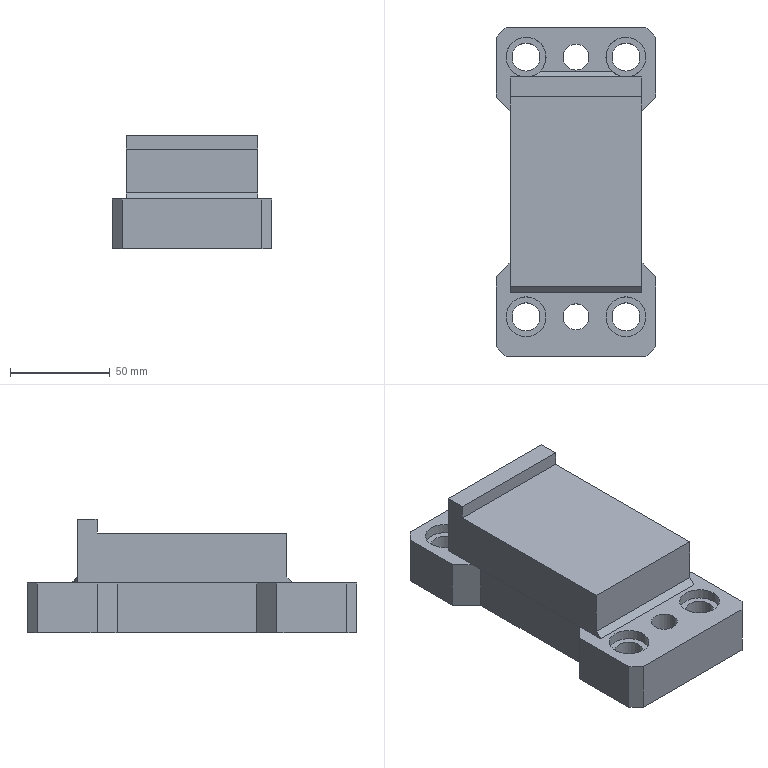Part | NX | features solid 2 | 1 solid | 44 faces | box 80 x 165 x 57 mm | volume 441871 mm3 | plane 34 | cylinder 10 | commonest cylinder face diameters 14 x4 20 x4 13 x2
STEP:
#1=CARTESIAN_POINT('',(-250.,-747.,-70.));
#2=VERTEX_POINT('',#1);
#3=CARTESIAN_POINT('',(-180.,-747.,-70.));
#4=VERTEX_POINT('',#3);
#5=CARTESIAN_POINT('',(-215.,-747.,-70.));
#6=DIRECTION('',(1.,0.,0.));
#7=VECTOR('',#6,1000.);
#8=LINE('',#5,#7);
#9=EDGE_CURVE('',#2,#4,#8,.T.);
#10=ORIENTED_EDGE('',*,*,#9,.T.);
#11=CARTESIAN_POINT('',(-175.,-742.,-70.));
#12=VERTEX_POINT('',#11);
#13=CARTESIAN_POINT('',(-156.25,-723.25,-70.));
#14=DIRECTION('',(0.7071,0.7071,0.));
#15=VECTOR('',#14,1000.);
#16=LINE('',#13,#15);
#17=EDGE_CURVE('',#12,#4,#16,.F.);
#18=ORIENTED_EDGE('',*,*,#17,.F.);
#19=CARTESIAN_POINT('',(-175.,-707.,-70.));
#20=VERTEX_POINT('',#19);
#21=CARTESIAN_POINT('',(-175.,-664.5,-70.));
#22=DIRECTION('',(0.,1.,0.));
#23=VECTOR('',#22,1000.);
#24=LINE('',#21,#23);
#25=EDGE_CURVE('',#12,#20,#24,.T.);
#26=ORIENTED_EDGE('',*,*,#25,.T.);
#27=CARTESIAN_POINT('',(-182.,-700.,-70.));
#28=VERTEX_POINT('',#27);
#29=CARTESIAN_POINT('',(-175.,-707.,-70.));
#30=DIRECTION('',(-0.7071,0.7071,0.));
#31=VECTOR('',#30,1000.);
#32=LINE('',#29,#31);
#33=EDGE_CURVE('',#20,#28,#32,.T.);
#34=ORIENTED_EDGE('',*,*,#33,.T.);
#35=CARTESIAN_POINT('',(-182.,-715.,-70.));
#36=VERTEX_POINT('',#35);
#37=CARTESIAN_POINT('',(-182.,-712.,-70.));
#38=DIRECTION('',(0.,1.,0.));
#39=VECTOR('',#38,1000.);
#40=LINE('',#37,#39);
#41=EDGE_CURVE('',#36,#28,#40,.T.);
#42=ORIENTED_EDGE('',*,*,#41,.F.);
#43=CARTESIAN_POINT('',(-248.,-715.,-70.));
#44=VERTEX_POINT('',#43);
#45=CARTESIAN_POINT('',(-182.,-715.,-70.));
#46=DIRECTION('',(1.,0.,0.));
#47=VECTOR('',#46,1000.);
#48=LINE('',#45,#47);
#49=EDGE_CURVE('',#44,#36,#48,.T.);
#50=ORIENTED_EDGE('',*,*,#49,.F.);
#51=CARTESIAN_POINT('',(-248.,-700.,-70.));
#52=VERTEX_POINT('',#51);
#53=CARTESIAN_POINT('',(-248.,-712.,-70.));
#54=DIRECTION('',(0.,1.,0.));
#55=VECTOR('',#54,1000.);
#56=LINE('',#53,#55);
#57=EDGE_CURVE('',#44,#52,#56,.T.);
#58=ORIENTED_EDGE('',*,*,#57,.T.);
#59=CARTESIAN_POINT('',(-255.,-707.,-70.));
#60=VERTEX_POINT('',#59);
#61=CARTESIAN_POINT('',(-245.,-697.,-70.));
#62=DIRECTION('',(-0.7071,-0.7071,0.));
#63=VECTOR('',#62,1000.);
#64=LINE('',#61,#63);
#65=EDGE_CURVE('',#52,#60,#64,.T.);
#66=ORIENTED_EDGE('',*,*,#65,.T.);
#67=CARTESIAN_POINT('',(-255.,-742.,-70.));
#68=VERTEX_POINT('',#67);
#69=CARTESIAN_POINT('',(-255.,-664.5,-70.));
#70=DIRECTION('',(0.,-1.,0.));
#71=VECTOR('',#70,1000.);
#72=LINE('',#69,#71);
#73=EDGE_CURVE('',#60,#68,#72,.T.);
#74=ORIENTED_EDGE('',*,*,#73,.T.);
#75=CARTESIAN_POINT('',(-273.75,-723.25,-70.));
#76=DIRECTION('',(0.7071,-0.7071,0.));
#77=VECTOR('',#76,1000.);
#78=LINE('',#75,#77);
#79=EDGE_CURVE('',#2,#68,#78,.F.);
#80=ORIENTED_EDGE('',*,*,#79,.F.);
#81=EDGE_LOOP('',(#10,#18,#26,#34,#42,#50,#58,#66,#74,#80));
#82=FACE_BOUND('',#81,.T.);
#83=CARTESIAN_POINT('',(-190.,-717.,-70.));
#84=VERTEX_POINT('',#83);
#85=CARTESIAN_POINT('',(-190.,-727.,-70.));
#86=DIRECTION('',(0.,0.,-1.));
#87=DIRECTION('',(0.,1.,0.));
#88=AXIS2_PLACEMENT_3D('',#85,#86,#87);
#89=CIRCLE('',#88,10.);
#90=EDGE_CURVE('',#84,#84,#89,.T.);
#91=ORIENTED_EDGE('',*,*,#90,.T.);
#92=EDGE_LOOP('',(#91));
#93=FACE_BOUND('',#92,.T.);
#94=CARTESIAN_POINT('',(-215.,-720.5,-70.));
#95=VERTEX_POINT('',#94);
#96=CARTESIAN_POINT('',(-215.,-727.,-70.));
#97=DIRECTION('',(0.,0.,-1.));
#98=DIRECTION('',(0.,1.,0.));
#99=AXIS2_PLACEMENT_3D('',#96,#97,#98);
#100=CIRCLE('',#99,6.5);
#101=EDGE_CURVE('',#95,#95,#100,.T.);
#102=ORIENTED_EDGE('',*,*,#101,.T.);
#103=EDGE_LOOP('',(#102));
#104=FACE_BOUND('',#103,.T.);
#105=CARTESIAN_POINT('',(-240.,-717.,-70.));
#106=VERTEX_POINT('',#105);
#107=CARTESIAN_POINT('',(-240.,-727.,-70.));
#108=DIRECTION('',(0.,0.,-1.));
#109=DIRECTION('',(0.,1.,0.));
#110=AXIS2_PLACEMENT_3D('',#107,#108,#109);
#111=CIRCLE('',#110,10.);
#112=EDGE_CURVE('',#106,#106,#111,.T.);
#113=ORIENTED_EDGE('',*,*,#112,.T.);
#114=EDGE_LOOP('',(#113));
#115=FACE_BOUND('',#114,.T.);
#116=CARTESIAN_POINT('',(-215.,-664.5,-70.));
#117=DIRECTION('',(0.,0.,1.));
#118=DIRECTION('',(0.,1.,0.));
#119=AXIS2_PLACEMENT_3D('',#116,#117,#118);
#120=PLANE('',#119);
#121=ADVANCED_FACE('',(#82,#93,#104,#115),#120,.T.);
#122=CARTESIAN_POINT('',(-180.,-582.,-70.));
#123=VERTEX_POINT('',#122);
#124=CARTESIAN_POINT('',(-250.,-582.,-70.));
#125=VERTEX_POINT('',#124);
#126=CARTESIAN_POINT('',(-215.,-582.,-70.));
#127=DIRECTION('',(-1.,0.,0.));
#128=VECTOR('',#127,1000.);
#129=LINE('',#126,#128);
#130=EDGE_CURVE('',#123,#125,#129,.T.);
#131=ORIENTED_EDGE('',*,*,#130,.T.);
#132=CARTESIAN_POINT('',(-255.,-587.,-70.));
#133=VERTEX_POINT('',#132);
#134=CARTESIAN_POINT('',(-273.75,-605.75,-70.));
#135=DIRECTION('',(-0.7071,-0.7071,0.));
#136=VECTOR('',#135,1000.);
#137=LINE('',#134,#136);
#138=EDGE_CURVE('',#133,#125,#137,.F.);
#139=ORIENTED_EDGE('',*,*,#138,.F.);
#140=CARTESIAN_POINT('',(-255.,-617.,-70.));
#141=VERTEX_POINT('',#140);
#142=CARTESIAN_POINT('',(-255.,-664.5,-70.));
#143=DIRECTION('',(0.,-1.,0.));
#144=VECTOR('',#143,1000.);
#145=LINE('',#142,#144);
#146=EDGE_CURVE('',#133,#141,#145,.T.);
#147=ORIENTED_EDGE('',*,*,#146,.T.);
#148=CARTESIAN_POINT('',(-248.,-624.,-70.));
#149=VERTEX_POINT('',#148);
#150=CARTESIAN_POINT('',(-245.,-627.,-70.));
#151=DIRECTION('',(-0.7071,0.7071,0.));
#152=VECTOR('',#151,1000.);
#153=LINE('',#150,#152);
#154=EDGE_CURVE('',#149,#141,#153,.T.);
#155=ORIENTED_EDGE('',*,*,#154,.F.);
#156=CARTESIAN_POINT('',(-248.,-607.,-70.));
#157=VERTEX_POINT('',#156);
#158=CARTESIAN_POINT('',(-248.,-712.,-70.));
#159=DIRECTION('',(0.,1.,0.));
#160=VECTOR('',#159,1000.);
#161=LINE('',#158,#160);
#162=EDGE_CURVE('',#149,#157,#161,.T.);
#163=ORIENTED_EDGE('',*,*,#162,.T.);
#164=CARTESIAN_POINT('',(-240.,-607.,-70.));
#165=VERTEX_POINT('',#164);
#166=CARTESIAN_POINT('',(-182.,-607.,-70.));
#167=DIRECTION('',(-1.,0.,0.));
#168=VECTOR('',#167,1000.);
#169=LINE('',#166,#168);
#170=EDGE_CURVE('',#165,#157,#169,.T.);
#171=ORIENTED_EDGE('',*,*,#170,.F.);
#172=CARTESIAN_POINT('',(-232.859,-604.,-70.));
#173=VERTEX_POINT('',#172);
#174=CARTESIAN_POINT('',(-240.,-597.,-70.));
#175=DIRECTION('',(0.,0.,-1.));
#176=DIRECTION('',(0.,1.,0.));
#177=AXIS2_PLACEMENT_3D('',#174,#175,#176);
#178=CIRCLE('',#177,10.);
#179=EDGE_CURVE('',#165,#173,#178,.T.);
#180=ORIENTED_EDGE('',*,*,#179,.T.);
#181=CARTESIAN_POINT('',(-197.141,-604.,-70.));
#182=VERTEX_POINT('',#181);
#183=CARTESIAN_POINT('',(-240.,-604.,-70.));
#184=DIRECTION('',(-1.,0.,0.));
#185=VECTOR('',#184,1000.);
#186=LINE('',#183,#185);
#187=EDGE_CURVE('',#182,#173,#186,.T.);
#188=ORIENTED_EDGE('',*,*,#187,.F.);
#189=CARTESIAN_POINT('',(-190.,-607.,-70.));
#190=VERTEX_POINT('',#189);
#191=CARTESIAN_POINT('',(-190.,-597.,-70.));
#192=DIRECTION('',(0.,0.,-1.));
#193=DIRECTION('',(0.,1.,0.));
#194=AXIS2_PLACEMENT_3D('',#191,#192,#193);
#195=CIRCLE('',#194,10.);
#196=EDGE_CURVE('',#182,#190,#195,.T.);
#197=ORIENTED_EDGE('',*,*,#196,.T.);
#198=CARTESIAN_POINT('',(-182.,-607.,-70.));
#199=VERTEX_POINT('',#198);
#200=CARTESIAN_POINT('',(-182.,-607.,-70.));
#201=DIRECTION('',(-1.,0.,0.));
#202=VECTOR('',#201,1000.);
#203=LINE('',#200,#202);
#204=EDGE_CURVE('',#199,#190,#203,.T.);
#205=ORIENTED_EDGE('',*,*,#204,.F.);
#206=CARTESIAN_POINT('',(-182.,-624.,-70.));
#207=VERTEX_POINT('',#206);
#208=CARTESIAN_POINT('',(-182.,-712.,-70.));
#209=DIRECTION('',(0.,1.,0.));
#210=VECTOR('',#209,1000.);
#211=LINE('',#208,#210);
#212=EDGE_CURVE('',#207,#199,#211,.T.);
#213=ORIENTED_EDGE('',*,*,#212,.F.);
#214=CARTESIAN_POINT('',(-175.,-617.,-70.));
#215=VERTEX_POINT('',#214);
#216=CARTESIAN_POINT('',(-175.,-617.,-70.));
#217=DIRECTION('',(-0.7071,-0.7071,0.));
#218=VECTOR('',#217,1000.);
#219=LINE('',#216,#218);
#220=EDGE_CURVE('',#215,#207,#219,.T.);
#221=ORIENTED_EDGE('',*,*,#220,.F.);
#222=CARTESIAN_POINT('',(-175.,-587.,-70.));
#223=VERTEX_POINT('',#222);
#224=CARTESIAN_POINT('',(-175.,-664.5,-70.));
#225=DIRECTION('',(0.,1.,0.));
#226=VECTOR('',#225,1000.);
#227=LINE('',#224,#226);
#228=EDGE_CURVE('',#215,#223,#227,.T.);
#229=ORIENTED_EDGE('',*,*,#228,.T.);
#230=CARTESIAN_POINT('',(-156.25,-605.75,-70.));
#231=DIRECTION('',(-0.7071,0.7071,0.));
#232=VECTOR('',#231,1000.);
#233=LINE('',#230,#232);
#234=EDGE_CURVE('',#123,#223,#233,.F.);
#235=ORIENTED_EDGE('',*,*,#234,.F.);
#236=EDGE_LOOP('',(#131,#139,#147,#155,#163,#171,#180,#188,#197,#205,#213,#221,#229,#235));
#237=FACE_BOUND('',#236,.T.);
#238=CARTESIAN_POINT('',(-215.,-590.5,-70.));
#239=VERTEX_POINT('',#238);
#240=CARTESIAN_POINT('',(-215.,-597.,-70.));
#241=DIRECTION('',(0.,0.,-1.));
#242=DIRECTION('',(0.,1.,0.));
#243=AXIS2_PLACEMENT_3D('',#240,#241,#242);
#244=CIRCLE('',#243,6.5);
#245=EDGE_CURVE('',#239,#239,#244,.T.);
#246=ORIENTED_EDGE('',*,*,#245,.T.);
#247=EDGE_LOOP('',(#246));
#248=FACE_BOUND('',#247,.T.);
#249=CARTESIAN_POINT('',(-215.,-664.5,-70.));
#250=DIRECTION('',(0.,0.,1.));
#251=DIRECTION('',(0.,1.,0.));
#252=AXIS2_PLACEMENT_3D('',#249,#250,#251);
#253=PLANE('',#252);
#254=ADVANCED_FACE('',(#237,#248),#253,.T.);
#255=CARTESIAN_POINT('',(-190.,-720.,-95.));
#256=VERTEX_POINT('',#255);
#257=CARTESIAN_POINT('',(-190.,-727.,-95.));
#258=DIRECTION('',(0.,0.,-1.));
#259=DIRECTION('',(0.,1.,0.));
#260=AXIS2_PLACEMENT_3D('',#257,#258,#259);
#261=CIRCLE('',#260,7.);
#262=EDGE_CURVE('',#256,#256,#261,.T.);
#263=ORIENTED_EDGE('',*,*,#262,.T.);
#264=EDGE_LOOP('',(#263));
#265=FACE_BOUND('',#264,.T.);
#266=CARTESIAN_POINT('',(-190.,-734.,-75.));
#267=VERTEX_POINT('',#266);
#268=CARTESIAN_POINT('',(-190.,-727.,-75.));
#269=DIRECTION('',(0.,0.,-1.));
#270=DIRECTION('',(0.,-1.,0.));
#271=AXIS2_PLACEMENT_3D('',#268,#269,#270);
#272=CIRCLE('',#271,7.);
#273=EDGE_CURVE('',#267,#267,#272,.T.);
#274=ORIENTED_EDGE('',*,*,#273,.F.);
#275=EDGE_LOOP('',(#274));
#276=FACE_BOUND('',#275,.T.);
#277=CARTESIAN_POINT('',(-190.,-727.,-70.));
#278=DIRECTION('',(0.,0.,-1.));
#279=DIRECTION('',(1.,0.,0.));
#280=AXIS2_PLACEMENT_3D('',#277,#278,#279);
#281=CYLINDRICAL_SURFACE('',#280,7.);
#282=ADVANCED_FACE('',(#265,#276),#281,.F.);
#283=CARTESIAN_POINT('',(-240.,-720.,-95.));
#284=VERTEX_POINT('',#283);
#285=CARTESIAN_POINT('',(-240.,-727.,-95.));
#286=DIRECTION('',(0.,0.,-1.));
#287=DIRECTION('',(0.,1.,0.));
#288=AXIS2_PLACEMENT_3D('',#285,#286,#287);
#289=CIRCLE('',#288,7.);
#290=EDGE_CURVE('',#284,#284,#289,.T.);
#291=ORIENTED_EDGE('',*,*,#290,.T.);
#292=EDGE_LOOP('',(#291));
#293=FACE_BOUND('',#292,.T.);
#294=CARTESIAN_POINT('',(-240.,-734.,-75.));
#295=VERTEX_POINT('',#294);
#296=CARTESIAN_POINT('',(-240.,-727.,-75.));
#297=DIRECTION('',(0.,0.,-1.));
#298=DIRECTION('',(0.,-1.,0.));
#299=AXIS2_PLACEMENT_3D('',#296,#297,#298);
#300=CIRCLE('',#299,7.);
#301=EDGE_CURVE('',#295,#295,#300,.T.);
#302=ORIENTED_EDGE('',*,*,#301,.F.);
#303=EDGE_LOOP('',(#302));
#304=FACE_BOUND('',#303,.T.);
#305=CARTESIAN_POINT('',(-240.,-727.,-70.));
#306=DIRECTION('',(0.,0.,-1.));
#307=DIRECTION('',(1.,0.,0.));
#308=AXIS2_PLACEMENT_3D('',#305,#306,#307);
#309=CYLINDRICAL_SURFACE('',#308,7.);
#310=ADVANCED_FACE('',(#293,#304),#309,.F.);
#311=CARTESIAN_POINT('',(-240.,-590.,-95.));
#312=VERTEX_POINT('',#311);
#313=CARTESIAN_POINT('',(-240.,-597.,-95.));
#314=DIRECTION('',(0.,0.,-1.));
#315=DIRECTION('',(0.,1.,0.));
#316=AXIS2_PLACEMENT_3D('',#313,#314,#315);
#317=CIRCLE('',#316,7.);
#318=EDGE_CURVE('',#312,#312,#317,.T.);
#319=ORIENTED_EDGE('',*,*,#318,.T.);
#320=EDGE_LOOP('',(#319));
#321=FACE_BOUND('',#320,.T.);
#322=CARTESIAN_POINT('',(-240.,-604.,-75.));
#323=VERTEX_POINT('',#322);
#324=CARTESIAN_POINT('',(-240.,-597.,-75.));
#325=DIRECTION('',(0.,0.,-1.));
#326=DIRECTION('',(0.,-1.,0.));
#327=AXIS2_PLACEMENT_3D('',#324,#325,#326);
#328=CIRCLE('',#327,7.);
#329=EDGE_CURVE('',#323,#323,#328,.T.);
#330=ORIENTED_EDGE('',*,*,#329,.F.);
#331=EDGE_LOOP('',(#330));
#332=FACE_BOUND('',#331,.T.);
#333=CARTESIAN_POINT('',(-240.,-597.,-70.));
#334=DIRECTION('',(0.,0.,-1.));
#335=DIRECTION('',(1.,0.,0.));
#336=AXIS2_PLACEMENT_3D('',#333,#334,#335);
#337=CYLINDRICAL_SURFACE('',#336,7.);
#338=ADVANCED_FACE('',(#321,#332),#337,.F.);
#339=CARTESIAN_POINT('',(-190.,-590.,-95.));
#340=VERTEX_POINT('',#339);
#341=CARTESIAN_POINT('',(-190.,-597.,-95.));
#342=DIRECTION('',(0.,0.,-1.));
#343=DIRECTION('',(0.,1.,0.));
#344=AXIS2_PLACEMENT_3D('',#341,#342,#343);
#345=CIRCLE('',#344,7.);
#346=EDGE_CURVE('',#340,#340,#345,.T.);
#347=ORIENTED_EDGE('',*,*,#346,.T.);
#348=EDGE_LOOP('',(#347));
#349=FACE_BOUND('',#348,.T.);
#350=CARTESIAN_POINT('',(-190.,-604.,-75.));
#351=VERTEX_POINT('',#350);
#352=CARTESIAN_POINT('',(-190.,-597.,-75.));
#353=DIRECTION('',(0.,0.,-1.));
#354=DIRECTION('',(0.,-1.,0.));
#355=AXIS2_PLACEMENT_3D('',#352,#353,#354);
#356=CIRCLE('',#355,7.);
#357=EDGE_CURVE('',#351,#351,#356,.T.);
#358=ORIENTED_EDGE('',*,*,#357,.F.);
#359=EDGE_LOOP('',(#358));
#360=FACE_BOUND('',#359,.T.);
#361=CARTESIAN_POINT('',(-190.,-597.,-70.));
#362=DIRECTION('',(0.,0.,-1.));
#363=DIRECTION('',(1.,0.,0.));
#364=AXIS2_PLACEMENT_3D('',#361,#362,#363);
#365=CYLINDRICAL_SURFACE('',#364,7.);
#366=ADVANCED_FACE('',(#349,#360),#365,.F.);
#367=CARTESIAN_POINT('',(-215.,-720.5,-95.));
#368=VERTEX_POINT('',#367);
#369=CARTESIAN_POINT('',(-215.,-727.,-95.));
#370=DIRECTION('',(0.,0.,-1.));
#371=DIRECTION('',(0.,1.,0.));
#372=AXIS2_PLACEMENT_3D('',#369,#370,#371);
#373=CIRCLE('',#372,6.5);
#374=EDGE_CURVE('',#368,#368,#373,.T.);
#375=ORIENTED_EDGE('',*,*,#374,.F.);
#376=EDGE_LOOP('',(#375));
#377=FACE_BOUND('',#376,.T.);
#378=ORIENTED_EDGE('',*,*,#318,.F.);
#379=EDGE_LOOP('',(#378));
#380=FACE_BOUND('',#379,.T.);
#381=ORIENTED_EDGE('',*,*,#346,.F.);
#382=EDGE_LOOP('',(#381));
#383=FACE_BOUND('',#382,.T.);
#384=CARTESIAN_POINT('',(-175.,-587.,-95.));
#385=VERTEX_POINT('',#384);
#386=CARTESIAN_POINT('',(-175.,-617.,-95.));
#387=VERTEX_POINT('',#386);
#388=CARTESIAN_POINT('',(-175.,-664.5,-95.));
#389=DIRECTION('',(0.,-1.,0.));
#390=VECTOR('',#389,1000.);
#391=LINE('',#388,#390);
#392=EDGE_CURVE('',#385,#387,#391,.T.);
#393=ORIENTED_EDGE('',*,*,#392,.T.);
#394=CARTESIAN_POINT('',(-185.,-627.,-95.));
#395=VERTEX_POINT('',#394);
#396=CARTESIAN_POINT('',(-175.,-617.,-95.));
#397=DIRECTION('',(-0.7071,-0.7071,0.));
#398=VECTOR('',#397,1000.);
#399=LINE('',#396,#398);
#400=EDGE_CURVE('',#387,#395,#399,.T.);
#401=ORIENTED_EDGE('',*,*,#400,.T.);
#402=CARTESIAN_POINT('',(-185.,-697.,-95.));
#403=VERTEX_POINT('',#402);
#404=CARTESIAN_POINT('',(-185.,-697.,-95.));
#405=DIRECTION('',(0.,1.,0.));
#406=VECTOR('',#405,1000.);
#407=LINE('',#404,#406);
#408=EDGE_CURVE('',#403,#395,#407,.T.);
#409=ORIENTED_EDGE('',*,*,#408,.F.);
#410=CARTESIAN_POINT('',(-175.,-707.,-95.));
#411=VERTEX_POINT('',#410);
#412=CARTESIAN_POINT('',(-175.,-707.,-95.));
#413=DIRECTION('',(-0.7071,0.7071,0.));
#414=VECTOR('',#413,1000.);
#415=LINE('',#412,#414);
#416=EDGE_CURVE('',#411,#403,#415,.T.);
#417=ORIENTED_EDGE('',*,*,#416,.F.);
#418=CARTESIAN_POINT('',(-175.,-742.,-95.));
#419=VERTEX_POINT('',#418);
#420=CARTESIAN_POINT('',(-175.,-664.5,-95.));
#421=DIRECTION('',(0.,-1.,0.));
#422=VECTOR('',#421,1000.);
#423=LINE('',#420,#422);
#424=EDGE_CURVE('',#411,#419,#423,.T.);
#425=ORIENTED_EDGE('',*,*,#424,.T.);
#426=CARTESIAN_POINT('',(-180.,-747.,-95.));
#427=VERTEX_POINT('',#426);
#428=CARTESIAN_POINT('',(-156.25,-723.25,-95.));
#429=DIRECTION('',(-0.7071,-0.7071,0.));
#430=VECTOR('',#429,1000.);
#431=LINE('',#428,#430);
#432=EDGE_CURVE('',#427,#419,#431,.F.);
#433=ORIENTED_EDGE('',*,*,#432,.F.);
#434=CARTESIAN_POINT('',(-250.,-747.,-95.));
#435=VERTEX_POINT('',#434);
#436=CARTESIAN_POINT('',(-215.,-747.,-95.));
#437=DIRECTION('',(-1.,0.,0.));
#438=VECTOR('',#437,1000.);
#439=LINE('',#436,#438);
#440=EDGE_CURVE('',#427,#435,#439,.T.);
#441=ORIENTED_EDGE('',*,*,#440,.T.);
#442=CARTESIAN_POINT('',(-255.,-742.,-95.));
#443=VERTEX_POINT('',#442);
#444=CARTESIAN_POINT('',(-273.75,-723.25,-95.));
#445=DIRECTION('',(-0.7071,0.7071,0.));
#446=VECTOR('',#445,1000.);
#447=LINE('',#444,#446);
#448=EDGE_CURVE('',#443,#435,#447,.F.);
#449=ORIENTED_EDGE('',*,*,#448,.F.);
#450=CARTESIAN_POINT('',(-255.,-707.,-95.));
#451=VERTEX_POINT('',#450);
#452=CARTESIAN_POINT('',(-255.,-664.5,-95.));
#453=DIRECTION('',(0.,1.,0.));
#454=VECTOR('',#453,1000.);
#455=LINE('',#452,#454);
#456=EDGE_CURVE('',#443,#451,#455,.T.);
#457=ORIENTED_EDGE('',*,*,#456,.T.);
#458=CARTESIAN_POINT('',(-245.,-697.,-95.));
#459=VERTEX_POINT('',#458);
#460=CARTESIAN_POINT('',(-245.,-697.,-95.));
#461=DIRECTION('',(-0.7071,-0.7071,0.));
#462=VECTOR('',#461,1000.);
#463=LINE('',#460,#462);
#464=EDGE_CURVE('',#459,#451,#463,.T.);
#465=ORIENTED_EDGE('',*,*,#464,.F.);
#466=CARTESIAN_POINT('',(-245.,-627.,-95.));
#467=VERTEX_POINT('',#466);
#468=CARTESIAN_POINT('',(-245.,-697.,-95.));
#469=DIRECTION('',(0.,1.,0.));
#470=VECTOR('',#469,1000.);
#471=LINE('',#468,#470);
#472=EDGE_CURVE('',#459,#467,#471,.T.);
#473=ORIENTED_EDGE('',*,*,#472,.T.);
#474=CARTESIAN_POINT('',(-255.,-617.,-95.));
#475=VERTEX_POINT('',#474);
#476=CARTESIAN_POINT('',(-245.,-627.,-95.));
#477=DIRECTION('',(-0.7071,0.7071,0.));
#478=VECTOR('',#477,1000.);
#479=LINE('',#476,#478);
#480=EDGE_CURVE('',#467,#475,#479,.T.);
#481=ORIENTED_EDGE('',*,*,#480,.T.);
#482=CARTESIAN_POINT('',(-255.,-587.,-95.));
#483=VERTEX_POINT('',#482);
#484=CARTESIAN_POINT('',(-255.,-664.5,-95.));
#485=DIRECTION('',(0.,1.,0.));
#486=VECTOR('',#485,1000.);
#487=LINE('',#484,#486);
#488=EDGE_CURVE('',#475,#483,#487,.T.);
#489=ORIENTED_EDGE('',*,*,#488,.T.);
#490=CARTESIAN_POINT('',(-250.,-582.,-95.));
#491=VERTEX_POINT('',#490);
#492=CARTESIAN_POINT('',(-273.75,-605.75,-95.));
#493=DIRECTION('',(0.7071,0.7071,0.));
#494=VECTOR('',#493,1000.);
#495=LINE('',#492,#494);
#496=EDGE_CURVE('',#491,#483,#495,.F.);
#497=ORIENTED_EDGE('',*,*,#496,.F.);
#498=CARTESIAN_POINT('',(-180.,-582.,-95.));
#499=VERTEX_POINT('',#498);
#500=CARTESIAN_POINT('',(-215.,-582.,-95.));
#501=DIRECTION('',(1.,0.,0.));
#502=VECTOR('',#501,1000.);
#503=LINE('',#500,#502);
#504=EDGE_CURVE('',#491,#499,#503,.T.);
#505=ORIENTED_EDGE('',*,*,#504,.T.);
#506=CARTESIAN_POINT('',(-156.25,-605.75,-95.));
#507=DIRECTION('',(0.7071,-0.7071,0.));
#508=VECTOR('',#507,1000.);
#509=LINE('',#506,#508);
#510=EDGE_CURVE('',#385,#499,#509,.F.);
#511=ORIENTED_EDGE('',*,*,#510,.F.);
#512=EDGE_LOOP('',(#393,#401,#409,#417,#425,#433,#441,#449,#457,#465,#473,#481,#489,#497,#505,#511));
#513=FACE_BOUND('',#512,.T.);
#514=CARTESIAN_POINT('',(-215.,-590.5,-95.));
#515=VERTEX_POINT('',#514);
#516=CARTESIAN_POINT('',(-215.,-597.,-95.));
#517=DIRECTION('',(0.,0.,-1.));
#518=DIRECTION('',(0.,1.,0.));
#519=AXIS2_PLACEMENT_3D('',#516,#517,#518);
#520=CIRCLE('',#519,6.5);
#521=EDGE_CURVE('',#515,#515,#520,.T.);
#522=ORIENTED_EDGE('',*,*,#521,.F.);
#523=EDGE_LOOP('',(#522));
#524=FACE_BOUND('',#523,.T.);
#525=ORIENTED_EDGE('',*,*,#262,.F.);
#526=EDGE_LOOP('',(#525));
#527=FACE_BOUND('',#526,.T.);
#528=ORIENTED_EDGE('',*,*,#290,.F.);
#529=EDGE_LOOP('',(#528));
#530=FACE_BOUND('',#529,.T.);
#531=CARTESIAN_POINT('',(-215.,-664.5,-95.));
#532=DIRECTION('',(0.,0.,-1.));
#533=DIRECTION('',(0.,-1.,0.));
#534=AXIS2_PLACEMENT_3D('',#531,#532,#533);
#535=PLANE('',#534);
#536=ADVANCED_FACE('',(#377,#380,#383,#513,#524,#527,#530),#535,.T.);
#537=ORIENTED_EDGE('',*,*,#73,.F.);
#538=CARTESIAN_POINT('',(-255.,-707.,-70.));
#539=DIRECTION('',(0.,0.,-1.));
#540=VECTOR('',#539,1000.);
#541=LINE('',#538,#540);
#542=EDGE_CURVE('',#60,#451,#541,.T.);
#543=ORIENTED_EDGE('',*,*,#542,.T.);
#544=ORIENTED_EDGE('',*,*,#456,.F.);
#545=CARTESIAN_POINT('',(-255.,-742.,-95.));
#546=DIRECTION('',(0.,0.,-1.));
#547=VECTOR('',#546,1000.);
#548=LINE('',#545,#547);
#549=EDGE_CURVE('',#68,#443,#548,.T.);
#550=ORIENTED_EDGE('',*,*,#549,.F.);
#551=EDGE_LOOP('',(#537,#543,#544,#550));
#552=FACE_BOUND('',#551,.T.);
#553=CARTESIAN_POINT('',(-255.,-664.5,-95.));
#554=DIRECTION('',(-1.,0.,0.));
#555=DIRECTION('',(0.,0.,-1.));
#556=AXIS2_PLACEMENT_3D('',#553,#554,#555);
#557=PLANE('',#556);
#558=ADVANCED_FACE('',(#552),#557,.T.);
#559=ORIENTED_EDGE('',*,*,#424,.F.);
#560=CARTESIAN_POINT('',(-175.,-707.,-70.));
#561=DIRECTION('',(0.,0.,-1.));
#562=VECTOR('',#561,1000.);
#563=LINE('',#560,#562);
#564=EDGE_CURVE('',#20,#411,#563,.T.);
#565=ORIENTED_EDGE('',*,*,#564,.F.);
#566=ORIENTED_EDGE('',*,*,#25,.F.);
#567=CARTESIAN_POINT('',(-175.,-742.,-95.));
#568=DIRECTION('',(0.,0.,1.));
#569=VECTOR('',#568,1000.);
#570=LINE('',#567,#569);
#571=EDGE_CURVE('',#419,#12,#570,.T.);
#572=ORIENTED_EDGE('',*,*,#571,.F.);
#573=EDGE_LOOP('',(#559,#565,#566,#572));
#574=FACE_BOUND('',#573,.T.);
#575=CARTESIAN_POINT('',(-175.,-664.5,-95.));
#576=DIRECTION('',(1.,0.,0.));
#577=DIRECTION('',(0.,0.,1.));
#578=AXIS2_PLACEMENT_3D('',#575,#576,#577);
#579=PLANE('',#578);
#580=ADVANCED_FACE('',(#574),#579,.T.);
#581=ORIENTED_EDGE('',*,*,#488,.F.);
#582=CARTESIAN_POINT('',(-255.,-617.,-70.));
#583=DIRECTION('',(0.,0.,-1.));
#584=VECTOR('',#583,1000.);
#585=LINE('',#582,#584);
#586=EDGE_CURVE('',#141,#475,#585,.T.);
#587=ORIENTED_EDGE('',*,*,#586,.F.);
#588=ORIENTED_EDGE('',*,*,#146,.F.);
#589=CARTESIAN_POINT('',(-255.,-587.,-95.));
#590=DIRECTION('',(0.,0.,1.));
#591=VECTOR('',#590,1000.);
#592=LINE('',#589,#591);
#593=EDGE_CURVE('',#483,#133,#592,.T.);
#594=ORIENTED_EDGE('',*,*,#593,.F.);
#595=EDGE_LOOP('',(#581,#587,#588,#594));
#596=FACE_BOUND('',#595,.T.);
#597=CARTESIAN_POINT('',(-255.,-664.5,-95.));
#598=DIRECTION('',(-1.,0.,0.));
#599=DIRECTION('',(0.,0.,-1.));
#600=AXIS2_PLACEMENT_3D('',#597,#598,#599);
#601=PLANE('',#600);
#602=ADVANCED_FACE('',(#596),#601,.T.);
#603=ORIENTED_EDGE('',*,*,#440,.F.);
#604=CARTESIAN_POINT('',(-180.,-747.,-95.));
#605=DIRECTION('',(0.,0.,-1.));
#606=VECTOR('',#605,1000.);
#607=LINE('',#604,#606);
#608=EDGE_CURVE('',#4,#427,#607,.T.);
#609=ORIENTED_EDGE('',*,*,#608,.F.);
#610=ORIENTED_EDGE('',*,*,#9,.F.);
#611=CARTESIAN_POINT('',(-250.,-747.,-95.));
#612=DIRECTION('',(0.,0.,1.));
#613=VECTOR('',#612,1000.);
#614=LINE('',#611,#613);
#615=EDGE_CURVE('',#435,#2,#614,.T.);
#616=ORIENTED_EDGE('',*,*,#615,.F.);
#617=EDGE_LOOP('',(#603,#609,#610,#616));
#618=FACE_BOUND('',#617,.T.);
#619=CARTESIAN_POINT('',(-215.,-747.,-95.));
#620=DIRECTION('',(0.,-1.,0.));
#621=DIRECTION('',(0.,0.,1.));
#622=AXIS2_PLACEMENT_3D('',#619,#620,#621);
#623=PLANE('',#622);
#624=ADVANCED_FACE('',(#618),#623,.T.);
#625=ORIENTED_EDGE('',*,*,#228,.F.);
#626=CARTESIAN_POINT('',(-175.,-617.,-70.));
#627=DIRECTION('',(0.,0.,-1.));
#628=VECTOR('',#627,1000.);
#629=LINE('',#626,#628);
#630=EDGE_CURVE('',#215,#387,#629,.T.);
#631=ORIENTED_EDGE('',*,*,#630,.T.);
#632=ORIENTED_EDGE('',*,*,#392,.F.);
#633=CARTESIAN_POINT('',(-175.,-587.,-95.));
#634=DIRECTION('',(0.,0.,-1.));
#635=VECTOR('',#634,1000.);
#636=LINE('',#633,#635);
#637=EDGE_CURVE('',#223,#385,#636,.T.);
#638=ORIENTED_EDGE('',*,*,#637,.F.);
#639=EDGE_LOOP('',(#625,#631,#632,#638));
#640=FACE_BOUND('',#639,.T.);
#641=CARTESIAN_POINT('',(-175.,-664.5,-95.));
#642=DIRECTION('',(1.,0.,0.));
#643=DIRECTION('',(0.,0.,1.));
#644=AXIS2_PLACEMENT_3D('',#641,#642,#643);
#645=PLANE('',#644);
#646=ADVANCED_FACE('',(#640),#645,.T.);
#647=ORIENTED_EDGE('',*,*,#504,.F.);
#648=CARTESIAN_POINT('',(-250.,-582.,-95.));
#649=DIRECTION('',(0.,0.,-1.));
#650=VECTOR('',#649,1000.);
#651=LINE('',#648,#650);
#652=EDGE_CURVE('',#125,#491,#651,.T.);
#653=ORIENTED_EDGE('',*,*,#652,.F.);
#654=ORIENTED_EDGE('',*,*,#130,.F.);
#655=CARTESIAN_POINT('',(-180.,-582.,-95.));
#656=DIRECTION('',(0.,0.,1.));
#657=VECTOR('',#656,1000.);
#658=LINE('',#655,#657);
#659=EDGE_CURVE('',#499,#123,#658,.T.);
#660=ORIENTED_EDGE('',*,*,#659,.F.);
#661=EDGE_LOOP('',(#647,#653,#654,#660));
#662=FACE_BOUND('',#661,.T.);
#663=CARTESIAN_POINT('',(-215.,-582.,-95.));
#664=DIRECTION('',(0.,1.,0.));
#665=DIRECTION('',(0.,0.,-1.));
#666=AXIS2_PLACEMENT_3D('',#663,#664,#665);
#667=PLANE('',#666);
#668=ADVANCED_FACE('',(#662),#667,.T.);
#669=ORIENTED_EDGE('',*,*,#400,.F.);
#670=ORIENTED_EDGE('',*,*,#630,.F.);
#671=ORIENTED_EDGE('',*,*,#220,.T.);
#672=CARTESIAN_POINT('',(-185.,-627.,-70.));
#673=VERTEX_POINT('',#672);
#674=CARTESIAN_POINT('',(-175.,-617.,-70.));
#675=DIRECTION('',(-0.7071,-0.7071,0.));
#676=VECTOR('',#675,1000.);
#677=LINE('',#674,#676);
#678=EDGE_CURVE('',#207,#673,#677,.T.);
#679=ORIENTED_EDGE('',*,*,#678,.T.);
#680=CARTESIAN_POINT('',(-185.,-627.,-70.));
#681=DIRECTION('',(0.,0.,-1.));
#682=VECTOR('',#681,1000.);
#683=LINE('',#680,#682);
#684=EDGE_CURVE('',#673,#395,#683,.T.);
#685=ORIENTED_EDGE('',*,*,#684,.T.);
#686=EDGE_LOOP('',(#669,#670,#671,#679,#685));
#687=FACE_BOUND('',#686,.T.);
#688=CARTESIAN_POINT('',(-175.,-617.,-70.));
#689=DIRECTION('',(-0.7071,0.7071,0.));
#690=DIRECTION('',(0.7071,0.7071,0.));
#691=AXIS2_PLACEMENT_3D('',#688,#689,#690);
#692=PLANE('',#691);
#693=ADVANCED_FACE('',(#687),#692,.F.);
#694=ORIENTED_EDGE('',*,*,#408,.T.);
#695=ORIENTED_EDGE('',*,*,#684,.F.);
#696=CARTESIAN_POINT('',(-185.,-697.,-70.));
#697=VERTEX_POINT('',#696);
#698=CARTESIAN_POINT('',(-185.,-697.,-70.));
#699=DIRECTION('',(0.,1.,0.));
#700=VECTOR('',#699,1000.);
#701=LINE('',#698,#700);
#702=EDGE_CURVE('',#697,#673,#701,.T.);
#703=ORIENTED_EDGE('',*,*,#702,.F.);
#704=CARTESIAN_POINT('',(-185.,-697.,-70.));
#705=DIRECTION('',(0.,0.,-1.));
#706=VECTOR('',#705,1000.);
#707=LINE('',#704,#706);
#708=EDGE_CURVE('',#697,#403,#707,.T.);
#709=ORIENTED_EDGE('',*,*,#708,.T.);
#710=EDGE_LOOP('',(#694,#695,#703,#709));
#711=FACE_BOUND('',#710,.T.);
#712=CARTESIAN_POINT('',(-185.,-697.,-70.));
#713=DIRECTION('',(1.,0.,0.));
#714=DIRECTION('',(0.,-1.,0.));
#715=AXIS2_PLACEMENT_3D('',#712,#713,#714);
#716=PLANE('',#715);
#717=ADVANCED_FACE('',(#711),#716,.T.);
#718=ORIENTED_EDGE('',*,*,#416,.T.);
#719=ORIENTED_EDGE('',*,*,#708,.F.);
#720=CARTESIAN_POINT('',(-175.,-707.,-70.));
#721=DIRECTION('',(-0.7071,0.7071,0.));
#722=VECTOR('',#721,1000.);
#723=LINE('',#720,#722);
#724=EDGE_CURVE('',#28,#697,#723,.T.);
#725=ORIENTED_EDGE('',*,*,#724,.F.);
#726=ORIENTED_EDGE('',*,*,#33,.F.);
#727=ORIENTED_EDGE('',*,*,#564,.T.);
#728=EDGE_LOOP('',(#718,#719,#725,#726,#727));
#729=FACE_BOUND('',#728,.T.);
#730=CARTESIAN_POINT('',(-175.,-707.,-70.));
#731=DIRECTION('',(0.7071,0.7071,0.));
#732=DIRECTION('',(0.7071,-0.7071,0.));
#733=AXIS2_PLACEMENT_3D('',#730,#731,#732);
#734=PLANE('',#733);
#735=ADVANCED_FACE('',(#729),#734,.T.);
#736=ORIENTED_EDGE('',*,*,#480,.F.);
#737=CARTESIAN_POINT('',(-245.,-627.,-70.));
#738=VERTEX_POINT('',#737);
#739=CARTESIAN_POINT('',(-245.,-627.,-70.));
#740=DIRECTION('',(0.,0.,-1.));
#741=VECTOR('',#740,1000.);
#742=LINE('',#739,#741);
#743=EDGE_CURVE('',#738,#467,#742,.T.);
#744=ORIENTED_EDGE('',*,*,#743,.F.);
#745=CARTESIAN_POINT('',(-245.,-627.,-70.));
#746=DIRECTION('',(-0.7071,0.7071,0.));
#747=VECTOR('',#746,1000.);
#748=LINE('',#745,#747);
#749=EDGE_CURVE('',#738,#149,#748,.T.);
#750=ORIENTED_EDGE('',*,*,#749,.T.);
#751=ORIENTED_EDGE('',*,*,#154,.T.);
#752=ORIENTED_EDGE('',*,*,#586,.T.);
#753=EDGE_LOOP('',(#736,#744,#750,#751,#752));
#754=FACE_BOUND('',#753,.T.);
#755=CARTESIAN_POINT('',(-245.,-627.,-70.));
#756=DIRECTION('',(0.7071,0.7071,0.));
#757=DIRECTION('',(0.7071,-0.7071,0.));
#758=AXIS2_PLACEMENT_3D('',#755,#756,#757);
#759=PLANE('',#758);
#760=ADVANCED_FACE('',(#754),#759,.F.);
#761=ORIENTED_EDGE('',*,*,#464,.T.);
#762=ORIENTED_EDGE('',*,*,#542,.F.);
#763=ORIENTED_EDGE('',*,*,#65,.F.);
#764=CARTESIAN_POINT('',(-245.,-697.,-70.));
#765=VERTEX_POINT('',#764);
#766=CARTESIAN_POINT('',(-245.,-697.,-70.));
#767=DIRECTION('',(-0.7071,-0.7071,0.));
#768=VECTOR('',#767,1000.);
#769=LINE('',#766,#768);
#770=EDGE_CURVE('',#765,#52,#769,.T.);
#771=ORIENTED_EDGE('',*,*,#770,.F.);
#772=CARTESIAN_POINT('',(-245.,-697.,-70.));
#773=DIRECTION('',(0.,0.,-1.));
#774=VECTOR('',#773,1000.);
#775=LINE('',#772,#774);
#776=EDGE_CURVE('',#765,#459,#775,.T.);
#777=ORIENTED_EDGE('',*,*,#776,.T.);
#778=EDGE_LOOP('',(#761,#762,#763,#771,#777));
#779=FACE_BOUND('',#778,.T.);
#780=CARTESIAN_POINT('',(-245.,-697.,-70.));
#781=DIRECTION('',(-0.7071,0.7071,0.));
#782=DIRECTION('',(0.7071,0.7071,0.));
#783=AXIS2_PLACEMENT_3D('',#780,#781,#782);
#784=PLANE('',#783);
#785=ADVANCED_FACE('',(#779),#784,.T.);
#786=ORIENTED_EDGE('',*,*,#472,.F.);
#787=ORIENTED_EDGE('',*,*,#776,.F.);
#788=CARTESIAN_POINT('',(-245.,-697.,-70.));
#789=DIRECTION('',(0.,1.,0.));
#790=VECTOR('',#789,1000.);
#791=LINE('',#788,#790);
#792=EDGE_CURVE('',#765,#738,#791,.T.);
#793=ORIENTED_EDGE('',*,*,#792,.T.);
#794=ORIENTED_EDGE('',*,*,#743,.T.);
#795=EDGE_LOOP('',(#786,#787,#793,#794));
#796=FACE_BOUND('',#795,.T.);
#797=CARTESIAN_POINT('',(-245.,-697.,-70.));
#798=DIRECTION('',(1.,0.,0.));
#799=DIRECTION('',(0.,-1.,0.));
#800=AXIS2_PLACEMENT_3D('',#797,#798,#799);
#801=PLANE('',#800);
#802=ADVANCED_FACE('',(#796),#801,.F.);
#803=ORIENTED_EDGE('',*,*,#245,.F.);
#804=EDGE_LOOP('',(#803));
#805=FACE_BOUND('',#804,.T.);
#806=ORIENTED_EDGE('',*,*,#521,.T.);
#807=EDGE_LOOP('',(#806));
#808=FACE_BOUND('',#807,.T.);
#809=CARTESIAN_POINT('',(-215.,-597.,-70.));
#810=DIRECTION('',(0.,0.,-1.));
#811=DIRECTION('',(1.,0.,0.));
#812=AXIS2_PLACEMENT_3D('',#809,#810,#811);
#813=CYLINDRICAL_SURFACE('',#812,6.5);
#814=ADVANCED_FACE('',(#805,#808),#813,.F.);
#815=ORIENTED_EDGE('',*,*,#101,.F.);
#816=EDGE_LOOP('',(#815));
#817=FACE_BOUND('',#816,.T.);
#818=ORIENTED_EDGE('',*,*,#374,.T.);
#819=EDGE_LOOP('',(#818));
#820=FACE_BOUND('',#819,.T.);
#821=CARTESIAN_POINT('',(-215.,-727.,-70.));
#822=DIRECTION('',(0.,0.,-1.));
#823=DIRECTION('',(1.,0.,0.));
#824=AXIS2_PLACEMENT_3D('',#821,#822,#823);
#825=CYLINDRICAL_SURFACE('',#824,6.5);
#826=ADVANCED_FACE('',(#817,#820),#825,.F.);
#827=ORIENTED_EDGE('',*,*,#196,.F.);
#828=CARTESIAN_POINT('',(-190.,-607.,-67.));
#829=VERTEX_POINT('',#828);
#830=CARTESIAN_POINT('',(-190.,-597.,-77.));
#831=DIRECTION('',(0.,-0.7071,-0.7071));
#832=DIRECTION('',(0.,0.7071,-0.7071));
#833=AXIS2_PLACEMENT_3D('',#830,#831,#832);
#834=ELLIPSE('',#833,14.142,10.);
#835=EDGE_CURVE('',#829,#182,#834,.T.);
#836=ORIENTED_EDGE('',*,*,#835,.F.);
#837=CARTESIAN_POINT('',(-190.,-607.,-68.5));
#838=DIRECTION('',(0.,0.,-1.));
#839=VECTOR('',#838,1000.);
#840=LINE('',#837,#839);
#841=EDGE_CURVE('',#829,#190,#840,.T.);
#842=ORIENTED_EDGE('',*,*,#841,.T.);
#843=EDGE_LOOP('',(#827,#836,#842));
#844=FACE_BOUND('',#843,.T.);
#845=CARTESIAN_POINT('',(-190.,-587.,-75.));
#846=VERTEX_POINT('',#845);
#847=CARTESIAN_POINT('',(-190.,-597.,-75.));
#848=DIRECTION('',(0.,0.,-1.));
#849=DIRECTION('',(0.,1.,0.));
#850=AXIS2_PLACEMENT_3D('',#847,#848,#849);
#851=CIRCLE('',#850,10.);
#852=EDGE_CURVE('',#846,#846,#851,.T.);
#853=ORIENTED_EDGE('',*,*,#852,.T.);
#854=EDGE_LOOP('',(#853));
#855=FACE_BOUND('',#854,.T.);
#856=CARTESIAN_POINT('',(-190.,-597.,-70.));
#857=DIRECTION('',(0.,0.,-1.));
#858=DIRECTION('',(1.,0.,0.));
#859=AXIS2_PLACEMENT_3D('',#856,#857,#858);
#860=CYLINDRICAL_SURFACE('',#859,10.);
#861=ADVANCED_FACE('',(#844,#855),#860,.F.);
#862=ORIENTED_EDGE('',*,*,#357,.T.);
#863=EDGE_LOOP('',(#862));
#864=FACE_BOUND('',#863,.T.);
#865=ORIENTED_EDGE('',*,*,#852,.F.);
#866=EDGE_LOOP('',(#865));
#867=FACE_BOUND('',#866,.T.);
#868=CARTESIAN_POINT('',(-190.,-597.,-75.));
#869=DIRECTION('',(0.,0.,1.));
#870=DIRECTION('',(0.,-1.,0.));
#871=AXIS2_PLACEMENT_3D('',#868,#869,#870);
#872=PLANE('',#871);
#873=ADVANCED_FACE('',(#864,#867),#872,.T.);
#874=ORIENTED_EDGE('',*,*,#179,.F.);
#875=CARTESIAN_POINT('',(-240.,-607.,-67.));
#876=VERTEX_POINT('',#875);
#877=CARTESIAN_POINT('',(-240.,-607.,-68.5));
#878=DIRECTION('',(0.,0.,-1.));
#879=VECTOR('',#878,1000.);
#880=LINE('',#877,#879);
#881=EDGE_CURVE('',#165,#876,#880,.F.);
#882=ORIENTED_EDGE('',*,*,#881,.T.);
#883=CARTESIAN_POINT('',(-240.,-597.,-77.));
#884=DIRECTION('',(0.,-0.7071,-0.7071));
#885=DIRECTION('',(0.,0.7071,-0.7071));
#886=AXIS2_PLACEMENT_3D('',#883,#884,#885);
#887=ELLIPSE('',#886,14.142,10.);
#888=EDGE_CURVE('',#173,#876,#887,.T.);
#889=ORIENTED_EDGE('',*,*,#888,.F.);
#890=EDGE_LOOP('',(#874,#882,#889));
#891=FACE_BOUND('',#890,.T.);
#892=CARTESIAN_POINT('',(-240.,-587.,-75.));
#893=VERTEX_POINT('',#892);
#894=CARTESIAN_POINT('',(-240.,-597.,-75.));
#895=DIRECTION('',(0.,0.,-1.));
#896=DIRECTION('',(0.,1.,0.));
#897=AXIS2_PLACEMENT_3D('',#894,#895,#896);
#898=CIRCLE('',#897,10.);
#899=EDGE_CURVE('',#893,#893,#898,.T.);
#900=ORIENTED_EDGE('',*,*,#899,.T.);
#901=EDGE_LOOP('',(#900));
#902=FACE_BOUND('',#901,.T.);
#903=CARTESIAN_POINT('',(-240.,-597.,-70.));
#904=DIRECTION('',(0.,0.,-1.));
#905=DIRECTION('',(1.,0.,0.));
#906=AXIS2_PLACEMENT_3D('',#903,#904,#905);
#907=CYLINDRICAL_SURFACE('',#906,10.);
#908=ADVANCED_FACE('',(#891,#902),#907,.F.);
#909=ORIENTED_EDGE('',*,*,#329,.T.);
#910=EDGE_LOOP('',(#909));
#911=FACE_BOUND('',#910,.T.);
#912=ORIENTED_EDGE('',*,*,#899,.F.);
#913=EDGE_LOOP('',(#912));
#914=FACE_BOUND('',#913,.T.);
#915=CARTESIAN_POINT('',(-240.,-597.,-75.));
#916=DIRECTION('',(0.,0.,1.));
#917=DIRECTION('',(0.,-1.,0.));
#918=AXIS2_PLACEMENT_3D('',#915,#916,#917);
#919=PLANE('',#918);
#920=ADVANCED_FACE('',(#911,#914),#919,.T.);
#921=ORIENTED_EDGE('',*,*,#112,.F.);
#922=EDGE_LOOP('',(#921));
#923=FACE_BOUND('',#922,.T.);
#924=CARTESIAN_POINT('',(-240.,-717.,-75.));
#925=VERTEX_POINT('',#924);
#926=CARTESIAN_POINT('',(-240.,-727.,-75.));
#927=DIRECTION('',(0.,0.,-1.));
#928=DIRECTION('',(0.,1.,0.));
#929=AXIS2_PLACEMENT_3D('',#926,#927,#928);
#930=CIRCLE('',#929,10.);
#931=EDGE_CURVE('',#925,#925,#930,.T.);
#932=ORIENTED_EDGE('',*,*,#931,.T.);
#933=EDGE_LOOP('',(#932));
#934=FACE_BOUND('',#933,.T.);
#935=CARTESIAN_POINT('',(-240.,-727.,-70.));
#936=DIRECTION('',(0.,0.,-1.));
#937=DIRECTION('',(1.,0.,0.));
#938=AXIS2_PLACEMENT_3D('',#935,#936,#937);
#939=CYLINDRICAL_SURFACE('',#938,10.);
#940=ADVANCED_FACE('',(#923,#934),#939,.F.);
#941=ORIENTED_EDGE('',*,*,#301,.T.);
#942=EDGE_LOOP('',(#941));
#943=FACE_BOUND('',#942,.T.);
#944=ORIENTED_EDGE('',*,*,#931,.F.);
#945=EDGE_LOOP('',(#944));
#946=FACE_BOUND('',#945,.T.);
#947=CARTESIAN_POINT('',(-240.,-727.,-75.));
#948=DIRECTION('',(0.,0.,1.));
#949=DIRECTION('',(0.,-1.,0.));
#950=AXIS2_PLACEMENT_3D('',#947,#948,#949);
#951=PLANE('',#950);
#952=ADVANCED_FACE('',(#943,#946),#951,.T.);
#953=ORIENTED_EDGE('',*,*,#90,.F.);
#954=EDGE_LOOP('',(#953));
#955=FACE_BOUND('',#954,.T.);
#956=CARTESIAN_POINT('',(-190.,-717.,-75.));
#957=VERTEX_POINT('',#956);
#958=CARTESIAN_POINT('',(-190.,-727.,-75.));
#959=DIRECTION('',(0.,0.,-1.));
#960=DIRECTION('',(0.,1.,0.));
#961=AXIS2_PLACEMENT_3D('',#958,#959,#960);
#962=CIRCLE('',#961,10.);
#963=EDGE_CURVE('',#957,#957,#962,.T.);
#964=ORIENTED_EDGE('',*,*,#963,.T.);
#965=EDGE_LOOP('',(#964));
#966=FACE_BOUND('',#965,.T.);
#967=CARTESIAN_POINT('',(-190.,-727.,-70.));
#968=DIRECTION('',(0.,0.,-1.));
#969=DIRECTION('',(1.,0.,0.));
#970=AXIS2_PLACEMENT_3D('',#967,#968,#969);
#971=CYLINDRICAL_SURFACE('',#970,10.);
#972=ADVANCED_FACE('',(#955,#966),#971,.F.);
#973=ORIENTED_EDGE('',*,*,#273,.T.);
#974=EDGE_LOOP('',(#973));
#975=FACE_BOUND('',#974,.T.);
#976=ORIENTED_EDGE('',*,*,#963,.F.);
#977=EDGE_LOOP('',(#976));
#978=FACE_BOUND('',#977,.T.);
#979=CARTESIAN_POINT('',(-190.,-727.,-75.));
#980=DIRECTION('',(0.,0.,1.));
#981=DIRECTION('',(0.,-1.,0.));
#982=AXIS2_PLACEMENT_3D('',#979,#980,#981);
#983=PLANE('',#982);
#984=ADVANCED_FACE('',(#975,#978),#983,.T.);
#985=ORIENTED_EDGE('',*,*,#770,.T.);
#986=CARTESIAN_POINT('',(-248.,-712.,-70.));
#987=DIRECTION('',(0.,1.,0.));
#988=VECTOR('',#987,1000.);
#989=LINE('',#986,#988);
#990=EDGE_CURVE('',#52,#149,#989,.T.);
#991=ORIENTED_EDGE('',*,*,#990,.T.);
#992=ORIENTED_EDGE('',*,*,#749,.F.);
#993=ORIENTED_EDGE('',*,*,#792,.F.);
#994=EDGE_LOOP('',(#985,#991,#992,#993));
#995=FACE_BOUND('',#994,.T.);
#996=CARTESIAN_POINT('',(-182.,-712.,-70.));
#997=DIRECTION('',(0.,0.,-1.));
#998=DIRECTION('',(1.,0.,0.));
#999=AXIS2_PLACEMENT_3D('',#996,#997,#998);
#1000=PLANE('',#999);
#1001=ADVANCED_FACE('',(#995),#1000,.T.);
#1002=CARTESIAN_POINT('',(-248.,-712.,-45.));
#1003=VERTEX_POINT('',#1002);
#1004=CARTESIAN_POINT('',(-248.,-617.,-45.));
#1005=VERTEX_POINT('',#1004);
#1006=CARTESIAN_POINT('',(-248.,-712.,-45.));
#1007=DIRECTION('',(0.,1.,0.));
#1008=VECTOR('',#1007,1000.);
#1009=LINE('',#1006,#1008);
#1010=EDGE_CURVE('',#1003,#1005,#1009,.T.);
#1011=ORIENTED_EDGE('',*,*,#1010,.F.);
#1012=CARTESIAN_POINT('',(-182.,-712.,-45.));
#1013=VERTEX_POINT('',#1012);
#1014=CARTESIAN_POINT('',(-182.,-712.,-45.));
#1015=DIRECTION('',(-1.,0.,0.));
#1016=VECTOR('',#1015,1000.);
#1017=LINE('',#1014,#1016);
#1018=EDGE_CURVE('',#1013,#1003,#1017,.T.);
#1019=ORIENTED_EDGE('',*,*,#1018,.F.);
#1020=CARTESIAN_POINT('',(-182.,-617.,-45.));
#1021=VERTEX_POINT('',#1020);
#1022=CARTESIAN_POINT('',(-182.,-712.,-45.));
#1023=DIRECTION('',(0.,1.,0.));
#1024=VECTOR('',#1023,1000.);
#1025=LINE('',#1022,#1024);
#1026=EDGE_CURVE('',#1013,#1021,#1025,.T.);
#1027=ORIENTED_EDGE('',*,*,#1026,.T.);
#1028=CARTESIAN_POINT('',(-182.,-617.,-45.));
#1029=DIRECTION('',(-1.,0.,0.));
#1030=VECTOR('',#1029,1000.);
#1031=LINE('',#1028,#1030);
#1032=EDGE_CURVE('',#1021,#1005,#1031,.T.);
#1033=ORIENTED_EDGE('',*,*,#1032,.T.);
#1034=EDGE_LOOP('',(#1011,#1019,#1027,#1033));
#1035=FACE_BOUND('',#1034,.T.);
#1036=CARTESIAN_POINT('',(-182.,-712.,-45.));
#1037=DIRECTION('',(0.,0.,-1.));
#1038=DIRECTION('',(1.,0.,0.));
#1039=AXIS2_PLACEMENT_3D('',#1036,#1037,#1038);
#1040=PLANE('',#1039);
#1041=ADVANCED_FACE('',(#1035),#1040,.F.);
#1042=CARTESIAN_POINT('',(-248.,-617.,-38.));
#1043=VERTEX_POINT('',#1042);
#1044=CARTESIAN_POINT('',(-248.,-617.,-45.));
#1045=DIRECTION('',(0.,0.,1.));
#1046=VECTOR('',#1045,1000.);
#1047=LINE('',#1044,#1046);
#1048=EDGE_CURVE('',#1005,#1043,#1047,.T.);
#1049=ORIENTED_EDGE('',*,*,#1048,.F.);
#1050=ORIENTED_EDGE('',*,*,#1032,.F.);
#1051=CARTESIAN_POINT('',(-182.,-617.,-38.));
#1052=VERTEX_POINT('',#1051);
#1053=CARTESIAN_POINT('',(-182.,-617.,-45.));
#1054=DIRECTION('',(0.,0.,1.));
#1055=VECTOR('',#1054,1000.);
#1056=LINE('',#1053,#1055);
#1057=EDGE_CURVE('',#1021,#1052,#1056,.T.);
#1058=ORIENTED_EDGE('',*,*,#1057,.T.);
#1059=CARTESIAN_POINT('',(-182.,-617.,-38.));
#1060=DIRECTION('',(-1.,0.,0.));
#1061=VECTOR('',#1060,1000.);
#1062=LINE('',#1059,#1061);
#1063=EDGE_CURVE('',#1052,#1043,#1062,.T.);
#1064=ORIENTED_EDGE('',*,*,#1063,.T.);
#1065=EDGE_LOOP('',(#1049,#1050,#1058,#1064));
#1066=FACE_BOUND('',#1065,.T.);
#1067=CARTESIAN_POINT('',(-182.,-617.,-45.));
#1068=DIRECTION('',(0.,1.,0.));
#1069=DIRECTION('',(1.,0.,0.));
#1070=AXIS2_PLACEMENT_3D('',#1067,#1068,#1069);
#1071=PLANE('',#1070);
#1072=ADVANCED_FACE('',(#1066),#1071,.F.);
#1073=CARTESIAN_POINT('',(-248.,-607.,-38.));
#1074=VERTEX_POINT('',#1073);
#1075=CARTESIAN_POINT('',(-248.,-617.,-38.));
#1076=DIRECTION('',(0.,1.,0.));
#1077=VECTOR('',#1076,1000.);
#1078=LINE('',#1075,#1077);
#1079=EDGE_CURVE('',#1043,#1074,#1078,.T.);
#1080=ORIENTED_EDGE('',*,*,#1079,.F.);
#1081=ORIENTED_EDGE('',*,*,#1063,.F.);
#1082=CARTESIAN_POINT('',(-182.,-607.,-38.));
#1083=VERTEX_POINT('',#1082);
#1084=CARTESIAN_POINT('',(-182.,-617.,-38.));
#1085=DIRECTION('',(0.,1.,0.));
#1086=VECTOR('',#1085,1000.);
#1087=LINE('',#1084,#1086);
#1088=EDGE_CURVE('',#1052,#1083,#1087,.T.);
#1089=ORIENTED_EDGE('',*,*,#1088,.T.);
#1090=CARTESIAN_POINT('',(-182.,-607.,-38.));
#1091=DIRECTION('',(-1.,0.,0.));
#1092=VECTOR('',#1091,1000.);
#1093=LINE('',#1090,#1092);
#1094=EDGE_CURVE('',#1083,#1074,#1093,.T.);
#1095=ORIENTED_EDGE('',*,*,#1094,.T.);
#1096=EDGE_LOOP('',(#1080,#1081,#1089,#1095));
#1097=FACE_BOUND('',#1096,.T.);
#1098=CARTESIAN_POINT('',(-182.,-617.,-38.));
#1099=DIRECTION('',(0.,0.,-1.));
#1100=DIRECTION('',(1.,0.,0.));
#1101=AXIS2_PLACEMENT_3D('',#1098,#1099,#1100);
#1102=PLANE('',#1101);
#1103=ADVANCED_FACE('',(#1097),#1102,.F.);
#1104=ORIENTED_EDGE('',*,*,#170,.T.);
#1105=CARTESIAN_POINT('',(-248.,-607.,-70.));
#1106=DIRECTION('',(0.,0.,1.));
#1107=VECTOR('',#1106,1000.);
#1108=LINE('',#1105,#1107);
#1109=EDGE_CURVE('',#157,#1074,#1108,.T.);
#1110=ORIENTED_EDGE('',*,*,#1109,.T.);
#1111=ORIENTED_EDGE('',*,*,#1094,.F.);
#1112=CARTESIAN_POINT('',(-182.,-607.,-70.));
#1113=DIRECTION('',(0.,0.,1.));
#1114=VECTOR('',#1113,1000.);
#1115=LINE('',#1112,#1114);
#1116=EDGE_CURVE('',#199,#1083,#1115,.T.);
#1117=ORIENTED_EDGE('',*,*,#1116,.F.);
#1118=ORIENTED_EDGE('',*,*,#204,.T.);
#1119=ORIENTED_EDGE('',*,*,#841,.F.);
#1120=CARTESIAN_POINT('',(-190.,-607.,-67.));
#1121=DIRECTION('',(1.,0.,0.));
#1122=VECTOR('',#1121,1000.);
#1123=LINE('',#1120,#1122);
#1124=EDGE_CURVE('',#876,#829,#1123,.T.);
#1125=ORIENTED_EDGE('',*,*,#1124,.F.);
#1126=ORIENTED_EDGE('',*,*,#881,.F.);
#1127=EDGE_LOOP('',(#1104,#1110,#1111,#1117,#1118,#1119,#1125,#1126));
#1128=FACE_BOUND('',#1127,.T.);
#1129=CARTESIAN_POINT('',(-182.,-607.,-70.));
#1130=DIRECTION('',(0.,1.,0.));
#1131=DIRECTION('',(1.,0.,0.));
#1132=AXIS2_PLACEMENT_3D('',#1129,#1130,#1131);
#1133=PLANE('',#1132);
#1134=ADVANCED_FACE('',(#1128),#1133,.T.);
#1135=CARTESIAN_POINT('',(-182.,-712.,-70.));
#1136=DIRECTION('',(0.,1.,0.));
#1137=VECTOR('',#1136,1000.);
#1138=LINE('',#1135,#1137);
#1139=EDGE_CURVE('',#28,#207,#1138,.T.);
#1140=ORIENTED_EDGE('',*,*,#1139,.F.);
#1141=ORIENTED_EDGE('',*,*,#724,.T.);
#1142=ORIENTED_EDGE('',*,*,#702,.T.);
#1143=ORIENTED_EDGE('',*,*,#678,.F.);
#1144=EDGE_LOOP('',(#1140,#1141,#1142,#1143));
#1145=FACE_BOUND('',#1144,.T.);
#1146=CARTESIAN_POINT('',(-182.,-712.,-70.));
#1147=DIRECTION('',(0.,0.,-1.));
#1148=DIRECTION('',(1.,0.,0.));
#1149=AXIS2_PLACEMENT_3D('',#1146,#1147,#1148);
#1150=PLANE('',#1149);
#1151=ADVANCED_FACE('',(#1145),#1150,.T.);
#1152=CARTESIAN_POINT('',(-182.,-712.,-67.));
#1153=VERTEX_POINT('',#1152);
#1154=CARTESIAN_POINT('',(-182.,-712.,-45.));
#1155=DIRECTION('',(0.,0.,-1.));
#1156=VECTOR('',#1155,1000.);
#1157=LINE('',#1154,#1156);
#1158=EDGE_CURVE('',#1013,#1153,#1157,.T.);
#1159=ORIENTED_EDGE('',*,*,#1158,.F.);
#1160=ORIENTED_EDGE('',*,*,#1018,.T.);
#1161=CARTESIAN_POINT('',(-248.,-712.,-67.));
#1162=VERTEX_POINT('',#1161);
#1163=CARTESIAN_POINT('',(-248.,-712.,-45.));
#1164=DIRECTION('',(0.,0.,-1.));
#1165=VECTOR('',#1164,1000.);
#1166=LINE('',#1163,#1165);
#1167=EDGE_CURVE('',#1003,#1162,#1166,.T.);
#1168=ORIENTED_EDGE('',*,*,#1167,.T.);
#1169=CARTESIAN_POINT('',(-248.,-712.,-67.));
#1170=DIRECTION('',(-1.,0.,0.));
#1171=VECTOR('',#1170,1000.);
#1172=LINE('',#1169,#1171);
#1173=EDGE_CURVE('',#1153,#1162,#1172,.T.);
#1174=ORIENTED_EDGE('',*,*,#1173,.F.);
#1175=EDGE_LOOP('',(#1159,#1160,#1168,#1174));
#1176=FACE_BOUND('',#1175,.T.);
#1177=CARTESIAN_POINT('',(-182.,-712.,-45.));
#1178=DIRECTION('',(0.,-1.,0.));
#1179=DIRECTION('',(-1.,0.,0.));
#1180=AXIS2_PLACEMENT_3D('',#1177,#1178,#1179);
#1181=PLANE('',#1180);
#1182=ADVANCED_FACE('',(#1176),#1181,.T.);
#1183=ORIENTED_EDGE('',*,*,#1026,.F.);
#1184=ORIENTED_EDGE('',*,*,#1158,.T.);
#1185=CARTESIAN_POINT('',(-182.,-653.5,-8.5));
#1186=DIRECTION('',(0.,-0.7071,-0.7071));
#1187=VECTOR('',#1186,1000.);
#1188=LINE('',#1185,#1187);
#1189=EDGE_CURVE('',#36,#1153,#1188,.F.);
#1190=ORIENTED_EDGE('',*,*,#1189,.F.);
#1191=ORIENTED_EDGE('',*,*,#41,.T.);
#1192=ORIENTED_EDGE('',*,*,#1139,.T.);
#1193=ORIENTED_EDGE('',*,*,#212,.T.);
#1194=ORIENTED_EDGE('',*,*,#1116,.T.);
#1195=ORIENTED_EDGE('',*,*,#1088,.F.);
#1196=ORIENTED_EDGE('',*,*,#1057,.F.);
#1197=EDGE_LOOP('',(#1183,#1184,#1190,#1191,#1192,#1193,#1194,#1195,#1196));
#1198=FACE_BOUND('',#1197,.T.);
#1199=CARTESIAN_POINT('',(-182.,-617.,-45.));
#1200=DIRECTION('',(-1.,0.,0.));
#1201=DIRECTION('',(0.,1.,0.));
#1202=AXIS2_PLACEMENT_3D('',#1199,#1200,#1201);
#1203=PLANE('',#1202);
#1204=ADVANCED_FACE('',(#1198),#1203,.F.);
#1205=ORIENTED_EDGE('',*,*,#1010,.T.);
#1206=ORIENTED_EDGE('',*,*,#1048,.T.);
#1207=ORIENTED_EDGE('',*,*,#1079,.T.);
#1208=ORIENTED_EDGE('',*,*,#1109,.F.);
#1209=ORIENTED_EDGE('',*,*,#162,.F.);
#1210=ORIENTED_EDGE('',*,*,#990,.F.);
#1211=ORIENTED_EDGE('',*,*,#57,.F.);
#1212=CARTESIAN_POINT('',(-248.,-712.,-67.));
#1213=DIRECTION('',(0.,0.7071,0.7071));
#1214=VECTOR('',#1213,1000.);
#1215=LINE('',#1212,#1214);
#1216=EDGE_CURVE('',#1162,#44,#1215,.F.);
#1217=ORIENTED_EDGE('',*,*,#1216,.F.);
#1218=ORIENTED_EDGE('',*,*,#1167,.F.);
#1219=EDGE_LOOP('',(#1205,#1206,#1207,#1208,#1209,#1210,#1211,#1217,#1218));
#1220=FACE_BOUND('',#1219,.T.);
#1221=CARTESIAN_POINT('',(-248.,-617.,-45.));
#1222=DIRECTION('',(-1.,0.,0.));
#1223=DIRECTION('',(0.,1.,0.));
#1224=AXIS2_PLACEMENT_3D('',#1221,#1222,#1223);
#1225=PLANE('',#1224);
#1226=ADVANCED_FACE('',(#1220),#1225,.T.);
#1227=ORIENTED_EDGE('',*,*,#1189,.T.);
#1228=ORIENTED_EDGE('',*,*,#1173,.T.);
#1229=ORIENTED_EDGE('',*,*,#1216,.T.);
#1230=ORIENTED_EDGE('',*,*,#49,.T.);
#1231=EDGE_LOOP('',(#1227,#1228,#1229,#1230));
#1232=FACE_BOUND('',#1231,.T.);
#1233=CARTESIAN_POINT('',(-182.,-712.,-67.));
#1234=DIRECTION('',(0.,-0.7071,0.7071));
#1235=DIRECTION('',(0.,-0.7071,-0.7071));
#1236=AXIS2_PLACEMENT_3D('',#1233,#1234,#1235);
#1237=PLANE('',#1236);
#1238=ADVANCED_FACE('',(#1232),#1237,.T.);
#1239=ORIENTED_EDGE('',*,*,#835,.T.);
#1240=ORIENTED_EDGE('',*,*,#187,.T.);
#1241=ORIENTED_EDGE('',*,*,#888,.T.);
#1242=ORIENTED_EDGE('',*,*,#1124,.T.);
#1243=EDGE_LOOP('',(#1239,#1240,#1241,#1242));
#1244=FACE_BOUND('',#1243,.T.);
#1245=CARTESIAN_POINT('',(-215.,-604.,-70.));
#1246=DIRECTION('',(0.,0.7071,0.7071));
#1247=DIRECTION('',(0.,-0.7071,0.7071));
#1248=AXIS2_PLACEMENT_3D('',#1245,#1246,#1247);
#1249=PLANE('',#1248);
#1250=ADVANCED_FACE('',(#1244),#1249,.T.);
#1251=ORIENTED_EDGE('',*,*,#234,.T.);
#1252=ORIENTED_EDGE('',*,*,#637,.T.);
#1253=ORIENTED_EDGE('',*,*,#510,.T.);
#1254=ORIENTED_EDGE('',*,*,#659,.T.);
#1255=EDGE_LOOP('',(#1251,#1252,#1253,#1254));
#1256=FACE_BOUND('',#1255,.T.);
#1257=CARTESIAN_POINT('',(-175.,-587.,-95.));
#1258=DIRECTION('',(-0.7071,-0.7071,0.));
#1259=DIRECTION('',(-0.7071,0.7071,0.));
#1260=AXIS2_PLACEMENT_3D('',#1257,#1258,#1259);
#1261=PLANE('',#1260);
#1262=ADVANCED_FACE('',(#1256),#1261,.F.);
#1263=ORIENTED_EDGE('',*,*,#138,.T.);
#1264=ORIENTED_EDGE('',*,*,#652,.T.);
#1265=ORIENTED_EDGE('',*,*,#496,.T.);
#1266=ORIENTED_EDGE('',*,*,#593,.T.);
#1267=EDGE_LOOP('',(#1263,#1264,#1265,#1266));
#1268=FACE_BOUND('',#1267,.T.);
#1269=CARTESIAN_POINT('',(-250.,-582.,-95.));
#1270=DIRECTION('',(0.7071,-0.7071,0.));
#1271=DIRECTION('',(-0.7071,-0.7071,0.));
#1272=AXIS2_PLACEMENT_3D('',#1269,#1270,#1271);
#1273=PLANE('',#1272);
#1274=ADVANCED_FACE('',(#1268),#1273,.F.);
#1275=ORIENTED_EDGE('',*,*,#79,.T.);
#1276=ORIENTED_EDGE('',*,*,#549,.T.);
#1277=ORIENTED_EDGE('',*,*,#448,.T.);
#1278=ORIENTED_EDGE('',*,*,#615,.T.);
#1279=EDGE_LOOP('',(#1275,#1276,#1277,#1278));
#1280=FACE_BOUND('',#1279,.T.);
#1281=CARTESIAN_POINT('',(-255.,-742.,-95.));
#1282=DIRECTION('',(0.7071,0.7071,0.));
#1283=DIRECTION('',(0.7071,-0.7071,0.));
#1284=AXIS2_PLACEMENT_3D('',#1281,#1282,#1283);
#1285=PLANE('',#1284);
#1286=ADVANCED_FACE('',(#1280),#1285,.F.);
#1287=ORIENTED_EDGE('',*,*,#17,.T.);
#1288=ORIENTED_EDGE('',*,*,#608,.T.);
#1289=ORIENTED_EDGE('',*,*,#432,.T.);
#1290=ORIENTED_EDGE('',*,*,#571,.T.);
#1291=EDGE_LOOP('',(#1287,#1288,#1289,#1290));
#1292=FACE_BOUND('',#1291,.T.);
#1293=CARTESIAN_POINT('',(-180.,-747.,-95.));
#1294=DIRECTION('',(-0.7071,0.7071,0.));
#1295=DIRECTION('',(0.7071,0.7071,0.));
#1296=AXIS2_PLACEMENT_3D('',#1293,#1294,#1295);
#1297=PLANE('',#1296);
#1298=ADVANCED_FACE('',(#1292),#1297,.F.);
#1299=CLOSED_SHELL('',(#121,#254,#282,#310,#338,#366,#536,#558,#580,#602,#624,#646,#668,#693,#717,#735,#760,#785,#802,#814,#826,#861,#873,#908,#920,#940,#952,#972,#984,#1001,#1041,#1072,#1103,#1134,#1151,#1182,#1204,#1226,#1238,#1250,#1262,#1274,#1286,#1298));
#1300=MANIFOLD_SOLID_BREP('',#1299);
#1301=(LENGTH_UNIT()NAMED_UNIT(*)SI_UNIT(.MILLI.,.METRE.));
#1302=UNCERTAINTY_MEASURE_WITH_UNIT(LENGTH_MEASURE(0.00001),#1301,'','');
#1303=(NAMED_UNIT(*)PLANE_ANGLE_UNIT()SI_UNIT($,.RADIAN.));
#1304=(NAMED_UNIT(*)SI_UNIT($,.STERADIAN.)SOLID_ANGLE_UNIT());
#1305=(GEOMETRIC_REPRESENTATION_CONTEXT(3)GLOBAL_UNCERTAINTY_ASSIGNED_CONTEXT((#1302))GLOBAL_UNIT_ASSIGNED_CONTEXT((#1301,#1303,#1304))REPRESENTATION_CONTEXT('',''));
#1306=ADVANCED_BREP_SHAPE_REPRESENTATION('',(#1300),#1305);